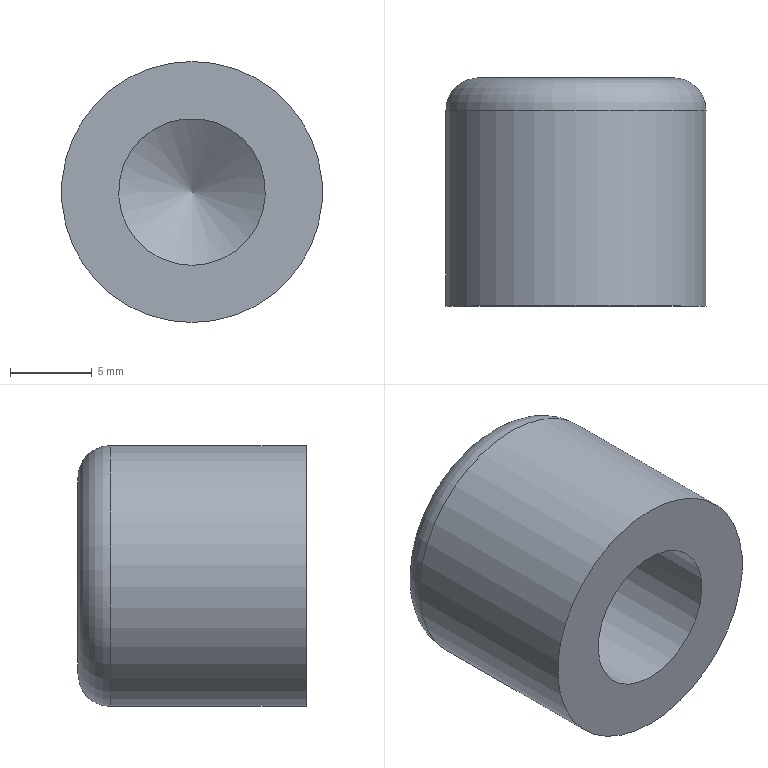Part | NX | 1 solid | 6 faces | box 16 x 14 x 16 mm | volume 2144 mm3 | cylinder 2 | plane 2 | cone 1 | torus 1 | commonest cylinder face diameters 9 x1 16 x1
STEP:
#1=CARTESIAN_POINT('',(0.,12.,8.));
#2=VERTEX_POINT('',#1);
#3=CARTESIAN_POINT('',(0.,12.,0.));
#4=DIRECTION('',(0.,1.,0.));
#5=DIRECTION('',(0.,0.,1.));
#6=AXIS2_PLACEMENT_3D('',#3,#4,#5);
#7=CIRCLE('',#6,8.);
#8=EDGE_CURVE('',#2,#2,#7,.F.);
#9=ORIENTED_EDGE('',*,*,#8,.T.);
#10=EDGE_LOOP('',(#9));
#11=FACE_BOUND('',#10,.T.);
#12=CARTESIAN_POINT('',(0.,0.,8.));
#13=VERTEX_POINT('',#12);
#14=CARTESIAN_POINT('',(0.,0.,0.));
#15=DIRECTION('',(0.,1.,0.));
#16=DIRECTION('',(0.,0.,1.));
#17=AXIS2_PLACEMENT_3D('',#14,#15,#16);
#18=CIRCLE('',#17,8.);
#19=EDGE_CURVE('',#13,#13,#18,.T.);
#20=ORIENTED_EDGE('',*,*,#19,.T.);
#21=EDGE_LOOP('',(#20));
#22=FACE_BOUND('',#21,.T.);
#23=CARTESIAN_POINT('',(0.,14.,0.));
#24=DIRECTION('',(0.,-1.,0.));
#25=DIRECTION('',(0.,0.,-1.));
#26=AXIS2_PLACEMENT_3D('',#23,#24,#25);
#27=CYLINDRICAL_SURFACE('',#26,8.);
#28=ADVANCED_FACE('',(#11,#22),#27,.T.);
#29=CARTESIAN_POINT('',(0.,14.,6.));
#30=VERTEX_POINT('',#29);
#31=CARTESIAN_POINT('',(0.,14.,0.));
#32=DIRECTION('',(0.,1.,0.));
#33=DIRECTION('',(0.,0.,1.));
#34=AXIS2_PLACEMENT_3D('',#31,#32,#33);
#35=CIRCLE('',#34,6.);
#36=EDGE_CURVE('',#30,#30,#35,.T.);
#37=ORIENTED_EDGE('',*,*,#36,.T.);
#38=EDGE_LOOP('',(#37));
#39=FACE_BOUND('',#38,.T.);
#40=CARTESIAN_POINT('',(0.,14.,0.));
#41=DIRECTION('',(0.,1.,0.));
#42=DIRECTION('',(0.,0.,1.));
#43=AXIS2_PLACEMENT_3D('',#40,#41,#42);
#44=PLANE('',#43);
#45=ADVANCED_FACE('',(#39),#44,.T.);
#46=CARTESIAN_POINT('',(0.,0.,-4.5));
#47=VERTEX_POINT('',#46);
#48=CARTESIAN_POINT('',(0.,0.,0.));
#49=DIRECTION('',(0.,-1.,0.));
#50=DIRECTION('',(0.,0.,-1.));
#51=AXIS2_PLACEMENT_3D('',#48,#49,#50);
#52=CIRCLE('',#51,4.5);
#53=EDGE_CURVE('',#47,#47,#52,.T.);
#54=ORIENTED_EDGE('',*,*,#53,.F.);
#55=EDGE_LOOP('',(#54));
#56=FACE_BOUND('',#55,.T.);
#57=ORIENTED_EDGE('',*,*,#19,.F.);
#58=EDGE_LOOP('',(#57));
#59=FACE_BOUND('',#58,.T.);
#60=CARTESIAN_POINT('',(0.,0.,0.));
#61=DIRECTION('',(0.,1.,0.));
#62=DIRECTION('',(0.,0.,1.));
#63=AXIS2_PLACEMENT_3D('',#60,#61,#62);
#64=PLANE('',#63);
#65=ADVANCED_FACE('',(#56,#59),#64,.F.);
#66=CARTESIAN_POINT('',(0.,11.704,0.));
#67=VERTEX_POINT('',#66);
#68=VERTEX_LOOP('',#67);
#69=FACE_BOUND('',#68,.T.);
#70=CARTESIAN_POINT('',(0.,9.,-4.5));
#71=VERTEX_POINT('',#70);
#72=CARTESIAN_POINT('',(0.,9.,0.));
#73=DIRECTION('',(0.,-1.,0.));
#74=DIRECTION('',(0.,0.,-1.));
#75=AXIS2_PLACEMENT_3D('',#72,#73,#74);
#76=CIRCLE('',#75,4.5);
#77=EDGE_CURVE('',#71,#71,#76,.T.);
#78=ORIENTED_EDGE('',*,*,#77,.T.);
#79=EDGE_LOOP('',(#78));
#80=FACE_BOUND('',#79,.T.);
#81=CARTESIAN_POINT('',(0.,9.,0.));
#82=DIRECTION('',(0.,-1.,0.));
#83=DIRECTION('',(0.,0.,-1.));
#84=AXIS2_PLACEMENT_3D('',#81,#82,#83);
#85=CONICAL_SURFACE('',#84,4.5,1.03);
#86=ADVANCED_FACE('',(#69,#80),#85,.F.);
#87=ORIENTED_EDGE('',*,*,#77,.F.);
#88=EDGE_LOOP('',(#87));
#89=FACE_BOUND('',#88,.T.);
#90=ORIENTED_EDGE('',*,*,#53,.T.);
#91=EDGE_LOOP('',(#90));
#92=FACE_BOUND('',#91,.T.);
#93=CARTESIAN_POINT('',(0.,0.,0.));
#94=DIRECTION('',(0.,-1.,0.));
#95=DIRECTION('',(0.,0.,-1.));
#96=AXIS2_PLACEMENT_3D('',#93,#94,#95);
#97=CYLINDRICAL_SURFACE('',#96,4.5);
#98=ADVANCED_FACE('',(#89,#92),#97,.F.);
#99=ORIENTED_EDGE('',*,*,#8,.F.);
#100=EDGE_LOOP('',(#99));
#101=FACE_BOUND('',#100,.T.);
#102=ORIENTED_EDGE('',*,*,#36,.F.);
#103=EDGE_LOOP('',(#102));
#104=FACE_BOUND('',#103,.T.);
#105=CARTESIAN_POINT('',(0.,12.,0.));
#106=DIRECTION('',(0.,1.,0.));
#107=DIRECTION('',(0.,0.,1.));
#108=AXIS2_PLACEMENT_3D('',#105,#106,#107);
#109=TOROIDAL_SURFACE('',#108,6.,2.);
#110=ADVANCED_FACE('',(#101,#104),#109,.T.);
#111=CLOSED_SHELL('',(#28,#45,#65,#86,#98,#110));
#112=MANIFOLD_SOLID_BREP('',#111);
#113=(LENGTH_UNIT()NAMED_UNIT(*)SI_UNIT(.MILLI.,.METRE.));
#114=UNCERTAINTY_MEASURE_WITH_UNIT(LENGTH_MEASURE(0.00001),#113,'','');
#115=(NAMED_UNIT(*)PLANE_ANGLE_UNIT()SI_UNIT($,.RADIAN.));
#116=(NAMED_UNIT(*)SI_UNIT($,.STERADIAN.)SOLID_ANGLE_UNIT());
#117=(GEOMETRIC_REPRESENTATION_CONTEXT(3)GLOBAL_UNCERTAINTY_ASSIGNED_CONTEXT((#114))GLOBAL_UNIT_ASSIGNED_CONTEXT((#113,#115,#116))REPRESENTATION_CONTEXT('',''));
#118=ADVANCED_BREP_SHAPE_REPRESENTATION('',(#112),#117);